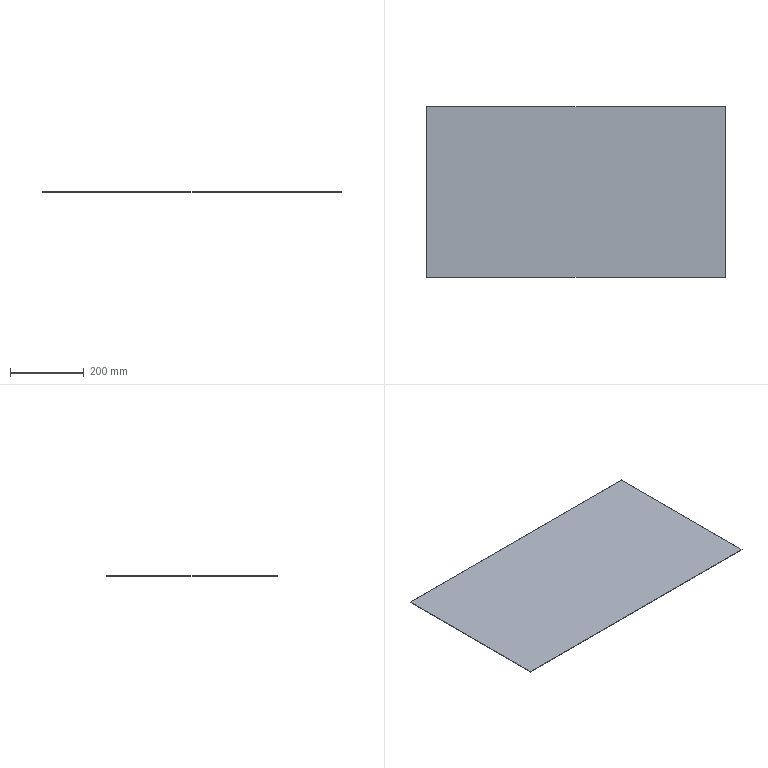Part | STEP file | Guide wheel mechanism revised.sldasm-Part-24 | 1 solid | 6 faces | box 810 x 461.99 x 1.2 mm | volume 449054 mm3 | plane 6
STEP:
#1=CARTESIAN_POINT('',(-405.,1428.01,505.));
#2=VERTEX_POINT('',#1);
#3=CARTESIAN_POINT('',(-405.,1890.,505.));
#4=VERTEX_POINT('',#3);
#5=CARTESIAN_POINT('',(-405.,1890.,505.));
#6=DIRECTION('',(0.,1.,0.));
#7=VECTOR('',#6,1000.);
#8=LINE('',#5,#7);
#9=EDGE_CURVE('',#2,#4,#8,.T.);
#10=ORIENTED_EDGE('',*,*,#9,.T.);
#11=CARTESIAN_POINT('',(-405.,1890.,503.8));
#12=VERTEX_POINT('',#11);
#13=CARTESIAN_POINT('',(-405.,1890.,503.8));
#14=DIRECTION('',(0.,0.,1.));
#15=VECTOR('',#14,1000.);
#16=LINE('',#13,#15);
#17=EDGE_CURVE('',#12,#4,#16,.T.);
#18=ORIENTED_EDGE('',*,*,#17,.F.);
#19=CARTESIAN_POINT('',(-405.,1428.01,503.8));
#20=VERTEX_POINT('',#19);
#21=CARTESIAN_POINT('',(-405.,1890.,503.8));
#22=DIRECTION('',(0.,1.,0.));
#23=VECTOR('',#22,1000.);
#24=LINE('',#21,#23);
#25=EDGE_CURVE('',#20,#12,#24,.T.);
#26=ORIENTED_EDGE('',*,*,#25,.F.);
#27=CARTESIAN_POINT('',(-405.,1428.01,503.8));
#28=DIRECTION('',(0.,0.,1.));
#29=VECTOR('',#28,1000.);
#30=LINE('',#27,#29);
#31=EDGE_CURVE('',#20,#2,#30,.T.);
#32=ORIENTED_EDGE('',*,*,#31,.T.);
#33=EDGE_LOOP('',(#10,#18,#26,#32));
#34=FACE_OUTER_BOUND('',#33,.T.);
#35=CARTESIAN_POINT('',(-405.,1890.,503.8));
#36=DIRECTION('',(1.,0.,0.));
#37=DIRECTION('',(0.,1.,0.));
#38=AXIS2_PLACEMENT_3D('',#35,#36,#37);
#39=PLANE('',#38);
#40=ADVANCED_FACE('',(#34),#39,.F.);
#41=CARTESIAN_POINT('',(405.,1890.,505.));
#42=VERTEX_POINT('',#41);
#43=CARTESIAN_POINT('',(-405.,1890.,505.));
#44=DIRECTION('',(1.,0.,0.));
#45=VECTOR('',#44,1000.);
#46=LINE('',#43,#45);
#47=EDGE_CURVE('',#4,#42,#46,.T.);
#48=ORIENTED_EDGE('',*,*,#47,.T.);
#49=CARTESIAN_POINT('',(405.,1890.,503.8));
#50=VERTEX_POINT('',#49);
#51=CARTESIAN_POINT('',(405.,1890.,503.8));
#52=DIRECTION('',(0.,0.,1.));
#53=VECTOR('',#52,1000.);
#54=LINE('',#51,#53);
#55=EDGE_CURVE('',#50,#42,#54,.T.);
#56=ORIENTED_EDGE('',*,*,#55,.F.);
#57=CARTESIAN_POINT('',(-405.,1890.,503.8));
#58=DIRECTION('',(1.,0.,0.));
#59=VECTOR('',#58,1000.);
#60=LINE('',#57,#59);
#61=EDGE_CURVE('',#12,#50,#60,.T.);
#62=ORIENTED_EDGE('',*,*,#61,.F.);
#63=ORIENTED_EDGE('',*,*,#17,.T.);
#64=EDGE_LOOP('',(#48,#56,#62,#63));
#65=FACE_OUTER_BOUND('',#64,.T.);
#66=CARTESIAN_POINT('',(-405.,1890.,503.8));
#67=DIRECTION('',(0.,-1.,0.));
#68=DIRECTION('',(0.,0.,-1.));
#69=AXIS2_PLACEMENT_3D('',#66,#67,#68);
#70=PLANE('',#69);
#71=ADVANCED_FACE('',(#65),#70,.F.);
#72=CARTESIAN_POINT('',(405.,1428.01,505.));
#73=VERTEX_POINT('',#72);
#74=CARTESIAN_POINT('',(405.,1890.,505.));
#75=DIRECTION('',(0.,-1.,0.));
#76=VECTOR('',#75,1000.);
#77=LINE('',#74,#76);
#78=EDGE_CURVE('',#42,#73,#77,.T.);
#79=ORIENTED_EDGE('',*,*,#78,.T.);
#80=CARTESIAN_POINT('',(405.,1428.01,503.8));
#81=VERTEX_POINT('',#80);
#82=CARTESIAN_POINT('',(405.,1428.01,503.8));
#83=DIRECTION('',(0.,0.,1.));
#84=VECTOR('',#83,1000.);
#85=LINE('',#82,#84);
#86=EDGE_CURVE('',#81,#73,#85,.T.);
#87=ORIENTED_EDGE('',*,*,#86,.F.);
#88=CARTESIAN_POINT('',(405.,1890.,503.8));
#89=DIRECTION('',(0.,-1.,0.));
#90=VECTOR('',#89,1000.);
#91=LINE('',#88,#90);
#92=EDGE_CURVE('',#50,#81,#91,.T.);
#93=ORIENTED_EDGE('',*,*,#92,.F.);
#94=ORIENTED_EDGE('',*,*,#55,.T.);
#95=EDGE_LOOP('',(#79,#87,#93,#94));
#96=FACE_OUTER_BOUND('',#95,.T.);
#97=CARTESIAN_POINT('',(405.,1890.,503.8));
#98=DIRECTION('',(-1.,0.,0.));
#99=DIRECTION('',(0.,-1.,0.));
#100=AXIS2_PLACEMENT_3D('',#97,#98,#99);
#101=PLANE('',#100);
#102=ADVANCED_FACE('',(#96),#101,.F.);
#103=CARTESIAN_POINT('',(-405.,1428.01,505.));
#104=DIRECTION('',(-1.,0.,0.));
#105=VECTOR('',#104,1000.);
#106=LINE('',#103,#105);
#107=EDGE_CURVE('',#73,#2,#106,.T.);
#108=ORIENTED_EDGE('',*,*,#107,.T.);
#109=ORIENTED_EDGE('',*,*,#31,.F.);
#110=CARTESIAN_POINT('',(-405.,1428.01,503.8));
#111=DIRECTION('',(-1.,0.,0.));
#112=VECTOR('',#111,1000.);
#113=LINE('',#110,#112);
#114=EDGE_CURVE('',#81,#20,#113,.T.);
#115=ORIENTED_EDGE('',*,*,#114,.F.);
#116=ORIENTED_EDGE('',*,*,#86,.T.);
#117=EDGE_LOOP('',(#108,#109,#115,#116));
#118=FACE_OUTER_BOUND('',#117,.T.);
#119=CARTESIAN_POINT('',(-405.,1428.01,503.8));
#120=DIRECTION('',(0.,1.,0.));
#121=DIRECTION('',(0.,0.,1.));
#122=AXIS2_PLACEMENT_3D('',#119,#120,#121);
#123=PLANE('',#122);
#124=ADVANCED_FACE('',(#118),#123,.F.);
#125=ORIENTED_EDGE('',*,*,#25,.T.);
#126=ORIENTED_EDGE('',*,*,#61,.T.);
#127=ORIENTED_EDGE('',*,*,#92,.T.);
#128=ORIENTED_EDGE('',*,*,#114,.T.);
#129=EDGE_LOOP('',(#125,#126,#127,#128));
#130=FACE_OUTER_BOUND('',#129,.T.);
#131=CARTESIAN_POINT('',(0.,0.,503.8));
#132=DIRECTION('',(0.,0.,1.));
#133=DIRECTION('',(1.,0.,0.));
#134=AXIS2_PLACEMENT_3D('',#131,#132,#133);
#135=PLANE('',#134);
#136=ADVANCED_FACE('',(#130),#135,.F.);
#137=ORIENTED_EDGE('',*,*,#9,.F.);
#138=ORIENTED_EDGE('',*,*,#107,.F.);
#139=ORIENTED_EDGE('',*,*,#78,.F.);
#140=ORIENTED_EDGE('',*,*,#47,.F.);
#141=EDGE_LOOP('',(#137,#138,#139,#140));
#142=FACE_OUTER_BOUND('',#141,.T.);
#143=CARTESIAN_POINT('',(0.,0.,505.));
#144=DIRECTION('',(0.,0.,1.));
#145=DIRECTION('',(1.,0.,0.));
#146=AXIS2_PLACEMENT_3D('',#143,#144,#145);
#147=PLANE('',#146);
#148=ADVANCED_FACE('',(#142),#147,.T.);
#149=CLOSED_SHELL('',(#40,#71,#102,#124,#136,#148));
#150=MANIFOLD_SOLID_BREP('',#149);
#151=CARTESIAN_POINT('',(0.,0.,0.));
#152=DIRECTION('',(0.,0.,1.));
#153=DIRECTION('',(1.,0.,0.));
#154=AXIS2_PLACEMENT_3D('',#151,#152,#153);
#155=(LENGTH_UNIT()NAMED_UNIT(*)SI_UNIT(.MILLI.,.METRE.));
#156=UNCERTAINTY_MEASURE_WITH_UNIT(LENGTH_MEASURE(0.00001),#155,'','');
#157=(NAMED_UNIT(*)PLANE_ANGLE_UNIT()SI_UNIT($,.RADIAN.));
#158=(NAMED_UNIT(*)SI_UNIT($,.STERADIAN.)SOLID_ANGLE_UNIT());
#159=(GEOMETRIC_REPRESENTATION_CONTEXT(3)GLOBAL_UNCERTAINTY_ASSIGNED_CONTEXT((#156))GLOBAL_UNIT_ASSIGNED_CONTEXT((#155,#157,#158))REPRESENTATION_CONTEXT('',''));
#160=ADVANCED_BREP_SHAPE_REPRESENTATION('',(#150,#154),#159);